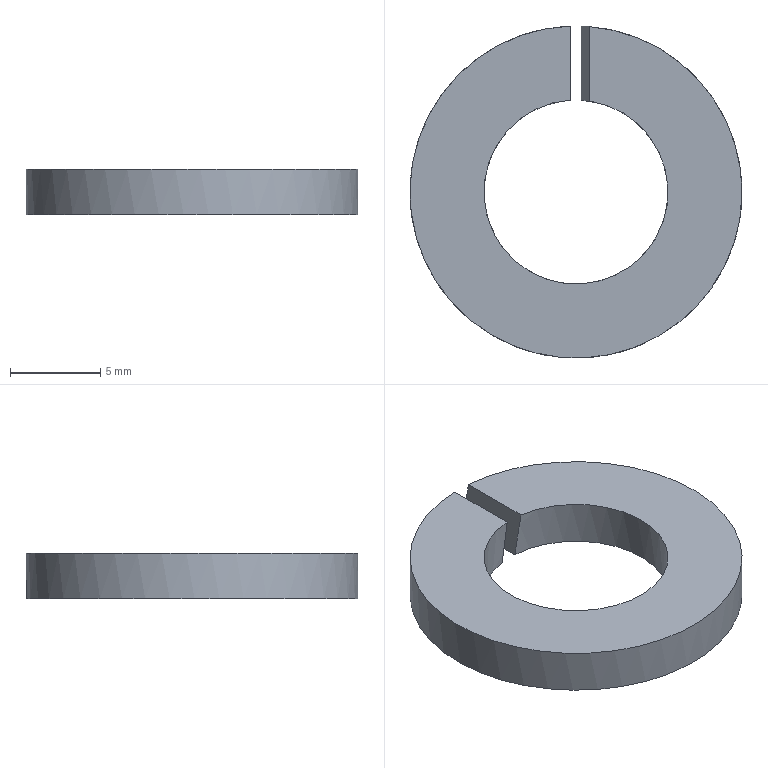Part | NX | features 5003_332_SLW10 2 | 1 solid | 6 faces | box 18.4 x 18.395 x 2.5 mm | volume 449.807 mm3 | plane 4 | cylinder 2 | commonest cylinder face diameters 10.2 x1 18.4 x1
STEP:
#1=CARTESIAN_POINT('',(258.825,42.195,-170.));
#2=VERTEX_POINT('',#1);
#3=CARTESIAN_POINT('',(258.825,38.091,-170.));
#4=VERTEX_POINT('',#3);
#5=CARTESIAN_POINT('',(258.825,42.2,-170.));
#6=DIRECTION('',(0.,-1.,0.));
#7=VECTOR('',#6,1000.);
#8=LINE('',#5,#7);
#9=EDGE_CURVE('',#2,#4,#8,.T.);
#10=ORIENTED_EDGE('',*,*,#9,.F.);
#11=CARTESIAN_POINT('',(257.785,42.17,-170.));
#12=VERTEX_POINT('',#11);
#13=CARTESIAN_POINT('',(258.525,33.,-170.));
#14=DIRECTION('',(0.,0.,-1.));
#15=DIRECTION('',(0.,1.,0.));
#16=AXIS2_PLACEMENT_3D('',#13,#14,#15);
#17=CIRCLE('',#16,9.2);
#18=EDGE_CURVE('',#2,#12,#17,.T.);
#19=ORIENTED_EDGE('',*,*,#18,.T.);
#20=CARTESIAN_POINT('',(257.785,38.046,-170.));
#21=VERTEX_POINT('',#20);
#22=CARTESIAN_POINT('',(257.785,42.2,-170.));
#23=DIRECTION('',(0.,-1.,0.));
#24=VECTOR('',#23,1000.);
#25=LINE('',#22,#24);
#26=EDGE_CURVE('',#12,#21,#25,.T.);
#27=ORIENTED_EDGE('',*,*,#26,.T.);
#28=CARTESIAN_POINT('',(258.525,33.,-170.));
#29=DIRECTION('',(0.,0.,-1.));
#30=DIRECTION('',(0.,1.,0.));
#31=AXIS2_PLACEMENT_3D('',#28,#29,#30);
#32=CIRCLE('',#31,5.1);
#33=EDGE_CURVE('',#4,#21,#32,.T.);
#34=ORIENTED_EDGE('',*,*,#33,.F.);
#35=EDGE_LOOP('',(#10,#19,#27,#34));
#36=FACE_BOUND('',#35,.T.);
#37=CARTESIAN_POINT('',(263.625,33.,-170.));
#38=DIRECTION('',(0.,0.,1.));
#39=DIRECTION('',(0.,-1.,0.));
#40=AXIS2_PLACEMENT_3D('',#37,#38,#39);
#41=PLANE('',#40);
#42=ADVANCED_FACE('',(#36),#41,.F.);
#43=CARTESIAN_POINT('',(259.265,42.17,-167.5));
#44=VERTEX_POINT('',#43);
#45=CARTESIAN_POINT('',(258.525,33.,-171.705));
#46=DIRECTION('',(-0.9849,0.,0.1733));
#47=DIRECTION('',(-0.1733,0.,-0.9849));
#48=AXIS2_PLACEMENT_3D('',#45,#46,#47);
#49=ELLIPSE('',#48,53.076,9.2);
#50=EDGE_CURVE('',#44,#2,#49,.T.);
#51=ORIENTED_EDGE('',*,*,#50,.F.);
#52=CARTESIAN_POINT('',(258.225,42.195,-167.5));
#53=VERTEX_POINT('',#52);
#54=CARTESIAN_POINT('',(258.525,33.,-167.5));
#55=DIRECTION('',(0.,0.,-1.));
#56=DIRECTION('',(0.,1.,0.));
#57=AXIS2_PLACEMENT_3D('',#54,#55,#56);
#58=CIRCLE('',#57,9.2);
#59=EDGE_CURVE('',#44,#53,#58,.T.);
#60=ORIENTED_EDGE('',*,*,#59,.T.);
#61=CARTESIAN_POINT('',(258.525,33.,-165.795));
#62=DIRECTION('',(0.9849,0.,-0.1733));
#63=DIRECTION('',(-0.1733,0.,-0.9849));
#64=AXIS2_PLACEMENT_3D('',#61,#62,#63);
#65=ELLIPSE('',#64,53.076,9.2);
#66=EDGE_CURVE('',#12,#53,#65,.T.);
#67=ORIENTED_EDGE('',*,*,#66,.F.);
#68=ORIENTED_EDGE('',*,*,#18,.F.);
#69=EDGE_LOOP('',(#51,#60,#67,#68));
#70=FACE_BOUND('',#69,.T.);
#71=CARTESIAN_POINT('',(258.525,33.,-170.));
#72=DIRECTION('',(0.,0.,-1.));
#73=DIRECTION('',(0.,1.,0.));
#74=AXIS2_PLACEMENT_3D('',#71,#72,#73);
#75=CYLINDRICAL_SURFACE('',#74,9.2);
#76=ADVANCED_FACE('',(#70),#75,.T.);
#77=CARTESIAN_POINT('',(259.265,38.046,-167.5));
#78=VERTEX_POINT('',#77);
#79=CARTESIAN_POINT('',(259.265,42.2,-167.5));
#80=DIRECTION('',(0.,-1.,0.));
#81=VECTOR('',#80,1000.);
#82=LINE('',#79,#81);
#83=EDGE_CURVE('',#44,#78,#82,.T.);
#84=ORIENTED_EDGE('',*,*,#83,.T.);
#85=CARTESIAN_POINT('',(258.225,38.091,-167.5));
#86=VERTEX_POINT('',#85);
#87=CARTESIAN_POINT('',(258.525,33.,-167.5));
#88=DIRECTION('',(0.,0.,-1.));
#89=DIRECTION('',(0.,1.,0.));
#90=AXIS2_PLACEMENT_3D('',#87,#88,#89);
#91=CIRCLE('',#90,5.1);
#92=EDGE_CURVE('',#78,#86,#91,.T.);
#93=ORIENTED_EDGE('',*,*,#92,.T.);
#94=CARTESIAN_POINT('',(258.225,42.2,-167.5));
#95=DIRECTION('',(0.,-1.,0.));
#96=VECTOR('',#95,1000.);
#97=LINE('',#94,#96);
#98=EDGE_CURVE('',#53,#86,#97,.T.);
#99=ORIENTED_EDGE('',*,*,#98,.F.);
#100=ORIENTED_EDGE('',*,*,#59,.F.);
#101=EDGE_LOOP('',(#84,#93,#99,#100));
#102=FACE_BOUND('',#101,.T.);
#103=CARTESIAN_POINT('',(263.625,33.,-167.5));
#104=DIRECTION('',(0.,0.,-1.));
#105=DIRECTION('',(0.,1.,0.));
#106=AXIS2_PLACEMENT_3D('',#103,#104,#105);
#107=PLANE('',#106);
#108=ADVANCED_FACE('',(#102),#107,.F.);
#109=CARTESIAN_POINT('',(258.525,33.,-171.705));
#110=DIRECTION('',(-0.9849,0.,0.1733));
#111=DIRECTION('',(-0.1733,0.,-0.9849));
#112=AXIS2_PLACEMENT_3D('',#109,#110,#111);
#113=ELLIPSE('',#112,29.423,5.1);
#114=EDGE_CURVE('',#4,#78,#113,.F.);
#115=ORIENTED_EDGE('',*,*,#114,.F.);
#116=ORIENTED_EDGE('',*,*,#33,.T.);
#117=CARTESIAN_POINT('',(258.525,33.,-165.795));
#118=DIRECTION('',(0.9849,0.,-0.1733));
#119=DIRECTION('',(-0.1733,0.,-0.9849));
#120=AXIS2_PLACEMENT_3D('',#117,#118,#119);
#121=ELLIPSE('',#120,29.423,5.1);
#122=EDGE_CURVE('',#86,#21,#121,.F.);
#123=ORIENTED_EDGE('',*,*,#122,.F.);
#124=ORIENTED_EDGE('',*,*,#92,.F.);
#125=EDGE_LOOP('',(#115,#116,#123,#124));
#126=FACE_BOUND('',#125,.T.);
#127=CARTESIAN_POINT('',(258.525,33.,-170.));
#128=DIRECTION('',(0.,0.,-1.));
#129=DIRECTION('',(0.,1.,0.));
#130=AXIS2_PLACEMENT_3D('',#127,#128,#129);
#131=CYLINDRICAL_SURFACE('',#130,5.1);
#132=ADVANCED_FACE('',(#126),#131,.F.);
#133=ORIENTED_EDGE('',*,*,#66,.T.);
#134=ORIENTED_EDGE('',*,*,#98,.T.);
#135=ORIENTED_EDGE('',*,*,#122,.T.);
#136=ORIENTED_EDGE('',*,*,#26,.F.);
#137=EDGE_LOOP('',(#133,#134,#135,#136));
#138=FACE_BOUND('',#137,.T.);
#139=CARTESIAN_POINT('',(257.785,42.2,-170.));
#140=DIRECTION('',(0.9849,0.,-0.1733));
#141=DIRECTION('',(-0.1733,0.,-0.9849));
#142=AXIS2_PLACEMENT_3D('',#139,#140,#141);
#143=PLANE('',#142);
#144=ADVANCED_FACE('',(#138),#143,.T.);
#145=ORIENTED_EDGE('',*,*,#50,.T.);
#146=ORIENTED_EDGE('',*,*,#9,.T.);
#147=ORIENTED_EDGE('',*,*,#114,.T.);
#148=ORIENTED_EDGE('',*,*,#83,.F.);
#149=EDGE_LOOP('',(#145,#146,#147,#148));
#150=FACE_BOUND('',#149,.T.);
#151=CARTESIAN_POINT('',(259.265,42.2,-167.5));
#152=DIRECTION('',(-0.9849,0.,0.1733));
#153=DIRECTION('',(0.1733,0.,0.9849));
#154=AXIS2_PLACEMENT_3D('',#151,#152,#153);
#155=PLANE('',#154);
#156=ADVANCED_FACE('',(#150),#155,.T.);
#157=CLOSED_SHELL('',(#42,#76,#108,#132,#144,#156));
#158=MANIFOLD_SOLID_BREP('',#157);
#159=(LENGTH_UNIT()NAMED_UNIT(*)SI_UNIT(.MILLI.,.METRE.));
#160=UNCERTAINTY_MEASURE_WITH_UNIT(LENGTH_MEASURE(0.00001),#159,'','');
#161=(NAMED_UNIT(*)PLANE_ANGLE_UNIT()SI_UNIT($,.RADIAN.));
#162=(NAMED_UNIT(*)SI_UNIT($,.STERADIAN.)SOLID_ANGLE_UNIT());
#163=(GEOMETRIC_REPRESENTATION_CONTEXT(3)GLOBAL_UNCERTAINTY_ASSIGNED_CONTEXT((#160))GLOBAL_UNIT_ASSIGNED_CONTEXT((#159,#161,#162))REPRESENTATION_CONTEXT('',''));
#164=ADVANCED_BREP_SHAPE_REPRESENTATION('',(#158),#163);